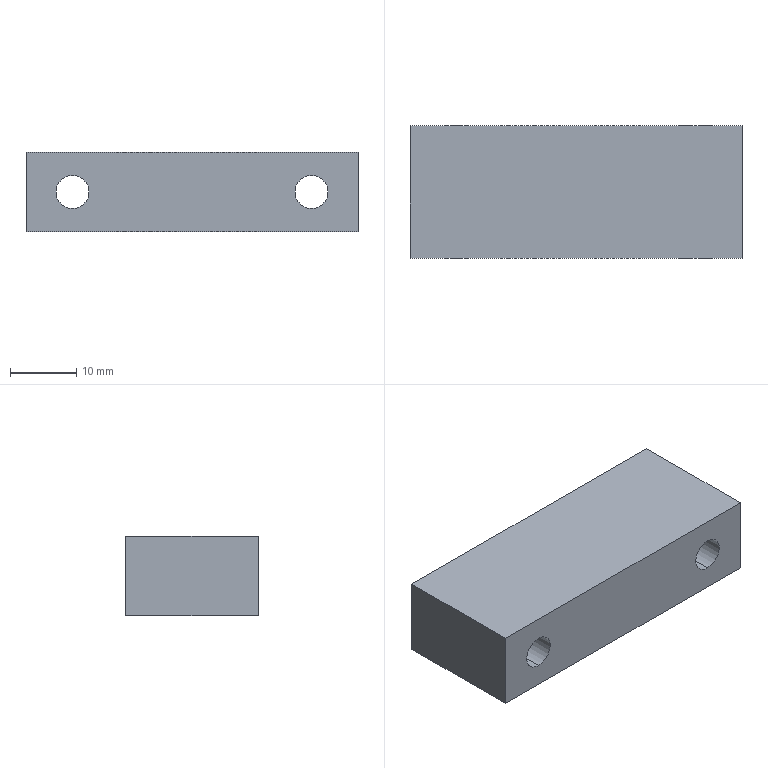Part | STEP file | Cylinder pad plate | 1 solid | 10 faces | box 50 x 20 x 12 mm | volume 11215 mm3 | plane 6 | cylinder 4 | commonest cylinder face diameters 5 x4
STEP:
#1=CARTESIAN_POINT('',(0.,0.,0.));
#2=DIRECTION('',(0.,0.,1.));
#3=DIRECTION('',(1.,0.,0.));
#4=AXIS2_PLACEMENT_3D('',#1,#2,#3);
#5=CARTESIAN_POINT('',(-137.752,17.174,8.5));
#6=VERTEX_POINT('',#5);
#7=CARTESIAN_POINT('',(-137.752,37.174,8.5));
#8=VERTEX_POINT('',#7);
#9=CARTESIAN_POINT('',(-137.752,17.174,8.5));
#10=DIRECTION('',(0.,1.,0.));
#11=VECTOR('',#10,1.);
#12=LINE('',#9,#11);
#13=CARTESIAN_POINT('',(-137.752,17.174,6.));
#14=DIRECTION('',(0.,1.,0.));
#15=DIRECTION('',(0.,0.,1.));
#16=AXIS2_PLACEMENT_3D('',#13,#14,#15);
#17=CYLINDRICAL_SURFACE('',#16,2.5);
#18=CARTESIAN_POINT('',(6.283,0.));
#19=DIRECTION('',(0.,1.));
#20=VECTOR('',#19,1.);
#21=LINE('',#18,#20);
#22=(GEOMETRIC_REPRESENTATION_CONTEXT(2)PARAMETRIC_REPRESENTATION_CONTEXT()REPRESENTATION_CONTEXT('',''));
#23=DEFINITIONAL_REPRESENTATION('',(#21),#22);
#24=PCURVE('',#17,#23);
#25=CARTESIAN_POINT('',(-137.752,17.174,6.));
#26=DIRECTION('',(0.,1.,0.));
#27=DIRECTION('',(0.,0.,1.));
#28=AXIS2_PLACEMENT_3D('',#25,#26,#27);
#29=CYLINDRICAL_SURFACE('',#28,2.5);
#30=CARTESIAN_POINT('',(0.,0.));
#31=DIRECTION('',(0.,1.));
#32=VECTOR('',#31,1.);
#33=LINE('',#30,#32);
#34=(GEOMETRIC_REPRESENTATION_CONTEXT(2)PARAMETRIC_REPRESENTATION_CONTEXT()REPRESENTATION_CONTEXT('',''));
#35=DEFINITIONAL_REPRESENTATION('',(#33),#34);
#36=PCURVE('',#29,#35);
#37=SURFACE_CURVE('',#12,(#24,#36),.PCURVE_S1.);
#38=EDGE_CURVE('',#6,#8,#37,.T.);
#39=ORIENTED_EDGE('',*,*,#38,.T.);
#40=CARTESIAN_POINT('',(-137.752,37.174,3.5));
#41=VERTEX_POINT('',#40);
#42=CARTESIAN_POINT('',(-137.752,37.174,6.));
#43=DIRECTION('',(0.,1.,0.));
#44=DIRECTION('',(0.,0.,1.));
#45=AXIS2_PLACEMENT_3D('',#42,#43,#44);
#46=CIRCLE('',#45,2.5);
#47=CARTESIAN_POINT('',(0.,20.));
#48=DIRECTION('',(1.,0.));
#49=VECTOR('',#48,1.);
#50=LINE('',#47,#49);
#51=(GEOMETRIC_REPRESENTATION_CONTEXT(2)PARAMETRIC_REPRESENTATION_CONTEXT()REPRESENTATION_CONTEXT('',''));
#52=DEFINITIONAL_REPRESENTATION('',(#50),#51);
#53=PCURVE('',#17,#52);
#54=CARTESIAN_POINT('',(-144.752,37.174,12.));
#55=DIRECTION('',(0.,-1.,0.));
#56=DIRECTION('',(0.,0.,-1.));
#57=AXIS2_PLACEMENT_3D('',#54,#55,#56);
#58=PLANE('',#57);
#59=CARTESIAN_POINT('',(3.5,7.));
#60=CARTESIAN_POINT('',(3.5,11.33));
#61=CARTESIAN_POINT('',(7.25,9.165));
#62=CARTESIAN_POINT('',(11.,7.));
#63=CARTESIAN_POINT('',(7.25,4.835));
#64=CARTESIAN_POINT('',(3.5,2.67));
#65=CARTESIAN_POINT('',(3.5,7.));
#66=(BOUNDED_CURVE()B_SPLINE_CURVE(2,(#59,#60,#61,#62,#63,#64,#65),.UNSPECIFIED.,.T.,.F.)B_SPLINE_CURVE_WITH_KNOTS((1,2,2,2,2,1),(-2.094,0.,2.094,4.189,6.283,8.378),.UNSPECIFIED.)CURVE()GEOMETRIC_REPRESENTATION_ITEM()RATIONAL_B_SPLINE_CURVE((1.,0.5,1.,0.5,1.,0.5,1.))REPRESENTATION_ITEM(''));
#67=(GEOMETRIC_REPRESENTATION_CONTEXT(2)PARAMETRIC_REPRESENTATION_CONTEXT()REPRESENTATION_CONTEXT('',''));
#68=DEFINITIONAL_REPRESENTATION('',(#66),#67);
#69=PCURVE('',#58,#68);
#70=SURFACE_CURVE('',#46,(#53,#69),.PCURVE_S1.);
#71=EDGE_CURVE('',#41,#8,#70,.T.);
#72=ORIENTED_EDGE('',*,*,#71,.F.);
#73=CARTESIAN_POINT('',(-137.752,17.174,3.5));
#74=VERTEX_POINT('',#73);
#75=CARTESIAN_POINT('',(-137.752,17.174,3.5));
#76=DIRECTION('',(0.,1.,0.));
#77=VECTOR('',#76,1.);
#78=LINE('',#75,#77);
#79=CARTESIAN_POINT('',(3.142,0.));
#80=DIRECTION('',(0.,1.));
#81=VECTOR('',#80,1.);
#82=LINE('',#79,#81);
#83=(GEOMETRIC_REPRESENTATION_CONTEXT(2)PARAMETRIC_REPRESENTATION_CONTEXT()REPRESENTATION_CONTEXT('',''));
#84=DEFINITIONAL_REPRESENTATION('',(#82),#83);
#85=PCURVE('',#17,#84);
#86=CARTESIAN_POINT('',(3.142,0.));
#87=DIRECTION('',(0.,1.));
#88=VECTOR('',#87,1.);
#89=LINE('',#86,#88);
#90=(GEOMETRIC_REPRESENTATION_CONTEXT(2)PARAMETRIC_REPRESENTATION_CONTEXT()REPRESENTATION_CONTEXT('',''));
#91=DEFINITIONAL_REPRESENTATION('',(#89),#90);
#92=PCURVE('',#29,#91);
#93=SURFACE_CURVE('',#78,(#85,#92),.PCURVE_S1.);
#94=EDGE_CURVE('',#74,#41,#93,.T.);
#95=ORIENTED_EDGE('',*,*,#94,.F.);
#96=CARTESIAN_POINT('',(-137.752,17.174,6.));
#97=DIRECTION('',(0.,1.,0.));
#98=DIRECTION('',(0.,0.,1.));
#99=AXIS2_PLACEMENT_3D('',#96,#97,#98);
#100=CIRCLE('',#99,2.5);
#101=CARTESIAN_POINT('',(0.,0.));
#102=DIRECTION('',(1.,0.));
#103=VECTOR('',#102,1.);
#104=LINE('',#101,#103);
#105=(GEOMETRIC_REPRESENTATION_CONTEXT(2)PARAMETRIC_REPRESENTATION_CONTEXT()REPRESENTATION_CONTEXT('',''));
#106=DEFINITIONAL_REPRESENTATION('',(#104),#105);
#107=PCURVE('',#17,#106);
#108=CARTESIAN_POINT('',(-144.752,17.174,12.));
#109=DIRECTION('',(0.,1.,0.));
#110=DIRECTION('',(0.,0.,1.));
#111=AXIS2_PLACEMENT_3D('',#108,#109,#110);
#112=PLANE('',#111);
#113=CARTESIAN_POINT('',(-6.,7.));
#114=DIRECTION('',(1.,0.));
#115=AXIS2_PLACEMENT_2D('',#113,#114);
#116=CIRCLE('',#115,2.5);
#117=(GEOMETRIC_REPRESENTATION_CONTEXT(2)PARAMETRIC_REPRESENTATION_CONTEXT()REPRESENTATION_CONTEXT('',''));
#118=DEFINITIONAL_REPRESENTATION('',(#116),#117);
#119=PCURVE('',#112,#118);
#120=SURFACE_CURVE('',#100,(#107,#119),.PCURVE_S1.);
#121=EDGE_CURVE('',#74,#6,#120,.T.);
#122=ORIENTED_EDGE('',*,*,#121,.T.);
#123=EDGE_LOOP('',(#39,#72,#95,#122));
#124=FACE_BOUND('',#123,.F.);
#125=ADVANCED_FACE('',(#124),#17,.F.);
#126=CARTESIAN_POINT('',(-101.752,17.174,8.5));
#127=VERTEX_POINT('',#126);
#128=CARTESIAN_POINT('',(-101.752,37.174,8.5));
#129=VERTEX_POINT('',#128);
#130=CARTESIAN_POINT('',(-101.752,17.174,8.5));
#131=DIRECTION('',(0.,1.,0.));
#132=VECTOR('',#131,1.);
#133=LINE('',#130,#132);
#134=CARTESIAN_POINT('',(-101.752,17.174,6.));
#135=DIRECTION('',(0.,1.,0.));
#136=DIRECTION('',(0.,0.,1.));
#137=AXIS2_PLACEMENT_3D('',#134,#135,#136);
#138=CYLINDRICAL_SURFACE('',#137,2.5);
#139=CARTESIAN_POINT('',(6.283,0.));
#140=DIRECTION('',(0.,1.));
#141=VECTOR('',#140,1.);
#142=LINE('',#139,#141);
#143=(GEOMETRIC_REPRESENTATION_CONTEXT(2)PARAMETRIC_REPRESENTATION_CONTEXT()REPRESENTATION_CONTEXT('',''));
#144=DEFINITIONAL_REPRESENTATION('',(#142),#143);
#145=PCURVE('',#138,#144);
#146=CARTESIAN_POINT('',(-101.752,17.174,6.));
#147=DIRECTION('',(0.,1.,0.));
#148=DIRECTION('',(0.,0.,1.));
#149=AXIS2_PLACEMENT_3D('',#146,#147,#148);
#150=CYLINDRICAL_SURFACE('',#149,2.5);
#151=CARTESIAN_POINT('',(0.,0.));
#152=DIRECTION('',(0.,1.));
#153=VECTOR('',#152,1.);
#154=LINE('',#151,#153);
#155=(GEOMETRIC_REPRESENTATION_CONTEXT(2)PARAMETRIC_REPRESENTATION_CONTEXT()REPRESENTATION_CONTEXT('',''));
#156=DEFINITIONAL_REPRESENTATION('',(#154),#155);
#157=PCURVE('',#150,#156);
#158=SURFACE_CURVE('',#133,(#145,#157),.PCURVE_S1.);
#159=EDGE_CURVE('',#127,#129,#158,.T.);
#160=ORIENTED_EDGE('',*,*,#159,.T.);
#161=CARTESIAN_POINT('',(-101.752,37.174,3.5));
#162=VERTEX_POINT('',#161);
#163=CARTESIAN_POINT('',(-101.752,37.174,6.));
#164=DIRECTION('',(0.,1.,0.));
#165=DIRECTION('',(0.,0.,1.));
#166=AXIS2_PLACEMENT_3D('',#163,#164,#165);
#167=CIRCLE('',#166,2.5);
#168=CARTESIAN_POINT('',(0.,20.));
#169=DIRECTION('',(1.,0.));
#170=VECTOR('',#169,1.);
#171=LINE('',#168,#170);
#172=(GEOMETRIC_REPRESENTATION_CONTEXT(2)PARAMETRIC_REPRESENTATION_CONTEXT()REPRESENTATION_CONTEXT('',''));
#173=DEFINITIONAL_REPRESENTATION('',(#171),#172);
#174=PCURVE('',#138,#173);
#175=CARTESIAN_POINT('',(3.5,43.));
#176=CARTESIAN_POINT('',(3.5,47.33));
#177=CARTESIAN_POINT('',(7.25,45.165));
#178=CARTESIAN_POINT('',(11.,43.));
#179=CARTESIAN_POINT('',(7.25,40.835));
#180=CARTESIAN_POINT('',(3.5,38.67));
#181=CARTESIAN_POINT('',(3.5,43.));
#182=(BOUNDED_CURVE()B_SPLINE_CURVE(2,(#175,#176,#177,#178,#179,#180,#181),.UNSPECIFIED.,.T.,.F.)B_SPLINE_CURVE_WITH_KNOTS((1,2,2,2,2,1),(-2.094,0.,2.094,4.189,6.283,8.378),.UNSPECIFIED.)CURVE()GEOMETRIC_REPRESENTATION_ITEM()RATIONAL_B_SPLINE_CURVE((1.,0.5,1.,0.5,1.,0.5,1.))REPRESENTATION_ITEM(''));
#183=(GEOMETRIC_REPRESENTATION_CONTEXT(2)PARAMETRIC_REPRESENTATION_CONTEXT()REPRESENTATION_CONTEXT('',''));
#184=DEFINITIONAL_REPRESENTATION('',(#182),#183);
#185=PCURVE('',#58,#184);
#186=SURFACE_CURVE('',#167,(#174,#185),.PCURVE_S1.);
#187=EDGE_CURVE('',#162,#129,#186,.T.);
#188=ORIENTED_EDGE('',*,*,#187,.F.);
#189=CARTESIAN_POINT('',(-101.752,17.174,3.5));
#190=VERTEX_POINT('',#189);
#191=CARTESIAN_POINT('',(-101.752,17.174,3.5));
#192=DIRECTION('',(0.,1.,0.));
#193=VECTOR('',#192,1.);
#194=LINE('',#191,#193);
#195=CARTESIAN_POINT('',(3.142,0.));
#196=DIRECTION('',(0.,1.));
#197=VECTOR('',#196,1.);
#198=LINE('',#195,#197);
#199=(GEOMETRIC_REPRESENTATION_CONTEXT(2)PARAMETRIC_REPRESENTATION_CONTEXT()REPRESENTATION_CONTEXT('',''));
#200=DEFINITIONAL_REPRESENTATION('',(#198),#199);
#201=PCURVE('',#138,#200);
#202=CARTESIAN_POINT('',(3.142,0.));
#203=DIRECTION('',(0.,1.));
#204=VECTOR('',#203,1.);
#205=LINE('',#202,#204);
#206=(GEOMETRIC_REPRESENTATION_CONTEXT(2)PARAMETRIC_REPRESENTATION_CONTEXT()REPRESENTATION_CONTEXT('',''));
#207=DEFINITIONAL_REPRESENTATION('',(#205),#206);
#208=PCURVE('',#150,#207);
#209=SURFACE_CURVE('',#194,(#201,#208),.PCURVE_S1.);
#210=EDGE_CURVE('',#190,#162,#209,.T.);
#211=ORIENTED_EDGE('',*,*,#210,.F.);
#212=CARTESIAN_POINT('',(-101.752,17.174,6.));
#213=DIRECTION('',(0.,1.,0.));
#214=DIRECTION('',(0.,0.,1.));
#215=AXIS2_PLACEMENT_3D('',#212,#213,#214);
#216=CIRCLE('',#215,2.5);
#217=CARTESIAN_POINT('',(0.,0.));
#218=DIRECTION('',(1.,0.));
#219=VECTOR('',#218,1.);
#220=LINE('',#217,#219);
#221=(GEOMETRIC_REPRESENTATION_CONTEXT(2)PARAMETRIC_REPRESENTATION_CONTEXT()REPRESENTATION_CONTEXT('',''));
#222=DEFINITIONAL_REPRESENTATION('',(#220),#221);
#223=PCURVE('',#138,#222);
#224=CARTESIAN_POINT('',(-6.,43.));
#225=DIRECTION('',(1.,0.));
#226=AXIS2_PLACEMENT_2D('',#224,#225);
#227=CIRCLE('',#226,2.5);
#228=(GEOMETRIC_REPRESENTATION_CONTEXT(2)PARAMETRIC_REPRESENTATION_CONTEXT()REPRESENTATION_CONTEXT('',''));
#229=DEFINITIONAL_REPRESENTATION('',(#227),#228);
#230=PCURVE('',#112,#229);
#231=SURFACE_CURVE('',#216,(#223,#230),.PCURVE_S1.);
#232=EDGE_CURVE('',#190,#127,#231,.T.);
#233=ORIENTED_EDGE('',*,*,#232,.T.);
#234=EDGE_LOOP('',(#160,#188,#211,#233));
#235=FACE_BOUND('',#234,.F.);
#236=ADVANCED_FACE('',(#235),#138,.F.);
#237=CARTESIAN_POINT('',(-94.752,17.174,0.));
#238=VERTEX_POINT('',#237);
#239=CARTESIAN_POINT('',(-94.752,37.174,0.));
#240=VERTEX_POINT('',#239);
#241=CARTESIAN_POINT('',(-94.752,17.174,0.));
#242=DIRECTION('',(0.,1.,0.));
#243=VECTOR('',#242,1.);
#244=LINE('',#241,#243);
#245=CARTESIAN_POINT('',(-94.752,17.174,12.));
#246=DIRECTION('',(-1.,0.,0.));
#247=DIRECTION('',(0.,-1.,0.));
#248=AXIS2_PLACEMENT_3D('',#245,#246,#247);
#249=PLANE('',#248);
#250=CARTESIAN_POINT('',(0.,-12.));
#251=DIRECTION('',(-1.,0.));
#252=VECTOR('',#251,1.);
#253=LINE('',#250,#252);
#254=(GEOMETRIC_REPRESENTATION_CONTEXT(2)PARAMETRIC_REPRESENTATION_CONTEXT()REPRESENTATION_CONTEXT('',''));
#255=DEFINITIONAL_REPRESENTATION('',(#253),#254);
#256=PCURVE('',#249,#255);
#257=CARTESIAN_POINT('',(0.,0.,0.));
#258=DIRECTION('',(0.,0.,-1.));
#259=DIRECTION('',(-1.,0.,0.));
#260=AXIS2_PLACEMENT_3D('',#257,#258,#259);
#261=PLANE('',#260);
#262=CARTESIAN_POINT('',(94.752,17.174));
#263=DIRECTION('',(0.,1.));
#264=VECTOR('',#263,1.);
#265=LINE('',#262,#264);
#266=(GEOMETRIC_REPRESENTATION_CONTEXT(2)PARAMETRIC_REPRESENTATION_CONTEXT()REPRESENTATION_CONTEXT('',''));
#267=DEFINITIONAL_REPRESENTATION('',(#265),#266);
#268=PCURVE('',#261,#267);
#269=SURFACE_CURVE('',#244,(#256,#268),.PCURVE_S1.);
#270=EDGE_CURVE('',#238,#240,#269,.T.);
#271=ORIENTED_EDGE('',*,*,#270,.T.);
#272=CARTESIAN_POINT('',(-94.752,37.174,12.));
#273=VERTEX_POINT('',#272);
#274=CARTESIAN_POINT('',(-94.752,37.174,12.));
#275=DIRECTION('',(0.,0.,-1.));
#276=VECTOR('',#275,1.);
#277=LINE('',#274,#276);
#278=CARTESIAN_POINT('',(-20.,0.));
#279=DIRECTION('',(0.,-1.));
#280=VECTOR('',#279,1.);
#281=LINE('',#278,#280);
#282=(GEOMETRIC_REPRESENTATION_CONTEXT(2)PARAMETRIC_REPRESENTATION_CONTEXT()REPRESENTATION_CONTEXT('',''));
#283=DEFINITIONAL_REPRESENTATION('',(#281),#282);
#284=PCURVE('',#249,#283);
#285=CARTESIAN_POINT('',(0.,50.));
#286=DIRECTION('',(1.,0.));
#287=VECTOR('',#286,1.);
#288=LINE('',#285,#287);
#289=(GEOMETRIC_REPRESENTATION_CONTEXT(2)PARAMETRIC_REPRESENTATION_CONTEXT()REPRESENTATION_CONTEXT('',''));
#290=DEFINITIONAL_REPRESENTATION('',(#288),#289);
#291=PCURVE('',#58,#290);
#292=SURFACE_CURVE('',#277,(#284,#291),.PCURVE_S1.);
#293=EDGE_CURVE('',#273,#240,#292,.T.);
#294=ORIENTED_EDGE('',*,*,#293,.F.);
#295=CARTESIAN_POINT('',(-94.752,17.174,12.));
#296=VERTEX_POINT('',#295);
#297=CARTESIAN_POINT('',(-94.752,17.174,12.));
#298=DIRECTION('',(0.,1.,0.));
#299=VECTOR('',#298,1.);
#300=LINE('',#297,#299);
#301=CARTESIAN_POINT('',(0.,0.));
#302=DIRECTION('',(-1.,0.));
#303=VECTOR('',#302,1.);
#304=LINE('',#301,#303);
#305=(GEOMETRIC_REPRESENTATION_CONTEXT(2)PARAMETRIC_REPRESENTATION_CONTEXT()REPRESENTATION_CONTEXT('',''));
#306=DEFINITIONAL_REPRESENTATION('',(#304),#305);
#307=PCURVE('',#249,#306);
#308=CARTESIAN_POINT('',(0.,0.,12.));
#309=DIRECTION('',(0.,0.,-1.));
#310=DIRECTION('',(-1.,0.,0.));
#311=AXIS2_PLACEMENT_3D('',#308,#309,#310);
#312=PLANE('',#311);
#313=CARTESIAN_POINT('',(94.752,17.174));
#314=DIRECTION('',(0.,1.));
#315=VECTOR('',#314,1.);
#316=LINE('',#313,#315);
#317=(GEOMETRIC_REPRESENTATION_CONTEXT(2)PARAMETRIC_REPRESENTATION_CONTEXT()REPRESENTATION_CONTEXT('',''));
#318=DEFINITIONAL_REPRESENTATION('',(#316),#317);
#319=PCURVE('',#312,#318);
#320=SURFACE_CURVE('',#300,(#307,#319),.PCURVE_S1.);
#321=EDGE_CURVE('',#296,#273,#320,.T.);
#322=ORIENTED_EDGE('',*,*,#321,.F.);
#323=CARTESIAN_POINT('',(-94.752,17.174,12.));
#324=DIRECTION('',(0.,0.,-1.));
#325=VECTOR('',#324,1.);
#326=LINE('',#323,#325);
#327=CARTESIAN_POINT('',(0.,0.));
#328=DIRECTION('',(0.,-1.));
#329=VECTOR('',#328,1.);
#330=LINE('',#327,#329);
#331=(GEOMETRIC_REPRESENTATION_CONTEXT(2)PARAMETRIC_REPRESENTATION_CONTEXT()REPRESENTATION_CONTEXT('',''));
#332=DEFINITIONAL_REPRESENTATION('',(#330),#331);
#333=PCURVE('',#249,#332);
#334=CARTESIAN_POINT('',(0.,50.));
#335=DIRECTION('',(-1.,0.));
#336=VECTOR('',#335,1.);
#337=LINE('',#334,#336);
#338=(GEOMETRIC_REPRESENTATION_CONTEXT(2)PARAMETRIC_REPRESENTATION_CONTEXT()REPRESENTATION_CONTEXT('',''));
#339=DEFINITIONAL_REPRESENTATION('',(#337),#338);
#340=PCURVE('',#112,#339);
#341=SURFACE_CURVE('',#326,(#333,#340),.PCURVE_S1.);
#342=EDGE_CURVE('',#296,#238,#341,.T.);
#343=ORIENTED_EDGE('',*,*,#342,.T.);
#344=EDGE_LOOP('',(#271,#294,#322,#343));
#345=FACE_BOUND('',#344,.T.);
#346=ADVANCED_FACE('',(#345),#249,.F.);
#347=CARTESIAN_POINT('',(-137.752,37.174,6.));
#348=DIRECTION('',(0.,1.,0.));
#349=DIRECTION('',(0.,0.,1.));
#350=AXIS2_PLACEMENT_3D('',#347,#348,#349);
#351=CIRCLE('',#350,2.5);
#352=CARTESIAN_POINT('',(3.5,7.));
#353=CARTESIAN_POINT('',(3.5,11.33));
#354=CARTESIAN_POINT('',(7.25,9.165));
#355=CARTESIAN_POINT('',(11.,7.));
#356=CARTESIAN_POINT('',(7.25,4.835));
#357=CARTESIAN_POINT('',(3.5,2.67));
#358=CARTESIAN_POINT('',(3.5,7.));
#359=(BOUNDED_CURVE()B_SPLINE_CURVE(2,(#352,#353,#354,#355,#356,#357,#358),.UNSPECIFIED.,.T.,.F.)B_SPLINE_CURVE_WITH_KNOTS((1,2,2,2,2,1),(-2.094,0.,2.094,4.189,6.283,8.378),.UNSPECIFIED.)CURVE()GEOMETRIC_REPRESENTATION_ITEM()RATIONAL_B_SPLINE_CURVE((1.,0.5,1.,0.5,1.,0.5,1.))REPRESENTATION_ITEM(''));
#360=(GEOMETRIC_REPRESENTATION_CONTEXT(2)PARAMETRIC_REPRESENTATION_CONTEXT()REPRESENTATION_CONTEXT('',''));
#361=DEFINITIONAL_REPRESENTATION('',(#359),#360);
#362=PCURVE('',#58,#361);
#363=CARTESIAN_POINT('',(0.,20.));
#364=DIRECTION('',(1.,0.));
#365=VECTOR('',#364,1.);
#366=LINE('',#363,#365);
#367=(GEOMETRIC_REPRESENTATION_CONTEXT(2)PARAMETRIC_REPRESENTATION_CONTEXT()REPRESENTATION_CONTEXT('',''));
#368=DEFINITIONAL_REPRESENTATION('',(#366),#367);
#369=PCURVE('',#29,#368);
#370=SURFACE_CURVE('',#351,(#362,#369),.PCURVE_S1.);
#371=EDGE_CURVE('',#8,#41,#370,.T.);
#372=ORIENTED_EDGE('',*,*,#371,.F.);
#373=ORIENTED_EDGE('',*,*,#71,.F.);
#374=EDGE_LOOP('',(#372,#373));
#375=FACE_BOUND('',#374,.T.);
#376=CARTESIAN_POINT('',(-101.752,37.174,6.));
#377=DIRECTION('',(0.,1.,0.));
#378=DIRECTION('',(0.,0.,1.));
#379=AXIS2_PLACEMENT_3D('',#376,#377,#378);
#380=CIRCLE('',#379,2.5);
#381=CARTESIAN_POINT('',(3.5,43.));
#382=CARTESIAN_POINT('',(3.5,47.33));
#383=CARTESIAN_POINT('',(7.25,45.165));
#384=CARTESIAN_POINT('',(11.,43.));
#385=CARTESIAN_POINT('',(7.25,40.835));
#386=CARTESIAN_POINT('',(3.5,38.67));
#387=CARTESIAN_POINT('',(3.5,43.));
#388=(BOUNDED_CURVE()B_SPLINE_CURVE(2,(#381,#382,#383,#384,#385,#386,#387),.UNSPECIFIED.,.T.,.F.)B_SPLINE_CURVE_WITH_KNOTS((1,2,2,2,2,1),(-2.094,0.,2.094,4.189,6.283,8.378),.UNSPECIFIED.)CURVE()GEOMETRIC_REPRESENTATION_ITEM()RATIONAL_B_SPLINE_CURVE((1.,0.5,1.,0.5,1.,0.5,1.))REPRESENTATION_ITEM(''));
#389=(GEOMETRIC_REPRESENTATION_CONTEXT(2)PARAMETRIC_REPRESENTATION_CONTEXT()REPRESENTATION_CONTEXT('',''));
#390=DEFINITIONAL_REPRESENTATION('',(#388),#389);
#391=PCURVE('',#58,#390);
#392=CARTESIAN_POINT('',(0.,20.));
#393=DIRECTION('',(1.,0.));
#394=VECTOR('',#393,1.);
#395=LINE('',#392,#394);
#396=(GEOMETRIC_REPRESENTATION_CONTEXT(2)PARAMETRIC_REPRESENTATION_CONTEXT()REPRESENTATION_CONTEXT('',''));
#397=DEFINITIONAL_REPRESENTATION('',(#395),#396);
#398=PCURVE('',#150,#397);
#399=SURFACE_CURVE('',#380,(#391,#398),.PCURVE_S1.);
#400=EDGE_CURVE('',#129,#162,#399,.T.);
#401=ORIENTED_EDGE('',*,*,#400,.F.);
#402=ORIENTED_EDGE('',*,*,#187,.F.);
#403=EDGE_LOOP('',(#401,#402));
#404=FACE_BOUND('',#403,.T.);
#405=CARTESIAN_POINT('',(-144.752,37.174,0.));
#406=VERTEX_POINT('',#405);
#407=CARTESIAN_POINT('',(-144.752,37.174,0.));
#408=DIRECTION('',(-1.,0.,0.));
#409=VECTOR('',#408,1.);
#410=LINE('',#407,#409);
#411=CARTESIAN_POINT('',(12.,0.));
#412=DIRECTION('',(0.,-1.));
#413=VECTOR('',#412,1.);
#414=LINE('',#411,#413);
#415=(GEOMETRIC_REPRESENTATION_CONTEXT(2)PARAMETRIC_REPRESENTATION_CONTEXT()REPRESENTATION_CONTEXT('',''));
#416=DEFINITIONAL_REPRESENTATION('',(#414),#415);
#417=PCURVE('',#58,#416);
#418=CARTESIAN_POINT('',(144.752,37.174));
#419=DIRECTION('',(1.,0.));
#420=VECTOR('',#419,1.);
#421=LINE('',#418,#420);
#422=(GEOMETRIC_REPRESENTATION_CONTEXT(2)PARAMETRIC_REPRESENTATION_CONTEXT()REPRESENTATION_CONTEXT('',''));
#423=DEFINITIONAL_REPRESENTATION('',(#421),#422);
#424=PCURVE('',#261,#423);
#425=SURFACE_CURVE('',#410,(#417,#424),.PCURVE_S1.);
#426=EDGE_CURVE('',#240,#406,#425,.T.);
#427=ORIENTED_EDGE('',*,*,#426,.T.);
#428=CARTESIAN_POINT('',(-144.752,37.174,12.));
#429=VERTEX_POINT('',#428);
#430=CARTESIAN_POINT('',(-144.752,37.174,12.));
#431=DIRECTION('',(0.,0.,-1.));
#432=VECTOR('',#431,1.);
#433=LINE('',#430,#432);
#434=CARTESIAN_POINT('',(0.,0.));
#435=DIRECTION('',(1.,0.));
#436=VECTOR('',#435,1.);
#437=LINE('',#434,#436);
#438=(GEOMETRIC_REPRESENTATION_CONTEXT(2)PARAMETRIC_REPRESENTATION_CONTEXT()REPRESENTATION_CONTEXT('',''));
#439=DEFINITIONAL_REPRESENTATION('',(#437),#438);
#440=PCURVE('',#58,#439);
#441=CARTESIAN_POINT('',(-144.752,17.174,12.));
#442=DIRECTION('',(1.,0.,0.));
#443=DIRECTION('',(0.,0.,-1.));
#444=AXIS2_PLACEMENT_3D('',#441,#442,#443);
#445=PLANE('',#444);
#446=CARTESIAN_POINT('',(0.,20.));
#447=DIRECTION('',(1.,0.));
#448=VECTOR('',#447,1.);
#449=LINE('',#446,#448);
#450=(GEOMETRIC_REPRESENTATION_CONTEXT(2)PARAMETRIC_REPRESENTATION_CONTEXT()REPRESENTATION_CONTEXT('',''));
#451=DEFINITIONAL_REPRESENTATION('',(#449),#450);
#452=PCURVE('',#445,#451);
#453=SURFACE_CURVE('',#433,(#440,#452),.PCURVE_S1.);
#454=EDGE_CURVE('',#429,#406,#453,.T.);
#455=ORIENTED_EDGE('',*,*,#454,.F.);
#456=CARTESIAN_POINT('',(-144.752,37.174,12.));
#457=DIRECTION('',(-1.,0.,0.));
#458=VECTOR('',#457,1.);
#459=LINE('',#456,#458);
#460=CARTESIAN_POINT('',(0.,0.));
#461=DIRECTION('',(0.,-1.));
#462=VECTOR('',#461,1.);
#463=LINE('',#460,#462);
#464=(GEOMETRIC_REPRESENTATION_CONTEXT(2)PARAMETRIC_REPRESENTATION_CONTEXT()REPRESENTATION_CONTEXT('',''));
#465=DEFINITIONAL_REPRESENTATION('',(#463),#464);
#466=PCURVE('',#58,#465);
#467=CARTESIAN_POINT('',(144.752,37.174));
#468=DIRECTION('',(1.,0.));
#469=VECTOR('',#468,1.);
#470=LINE('',#467,#469);
#471=(GEOMETRIC_REPRESENTATION_CONTEXT(2)PARAMETRIC_REPRESENTATION_CONTEXT()REPRESENTATION_CONTEXT('',''));
#472=DEFINITIONAL_REPRESENTATION('',(#470),#471);
#473=PCURVE('',#312,#472);
#474=SURFACE_CURVE('',#459,(#466,#473),.PCURVE_S1.);
#475=EDGE_CURVE('',#273,#429,#474,.T.);
#476=ORIENTED_EDGE('',*,*,#475,.F.);
#477=ORIENTED_EDGE('',*,*,#293,.T.);
#478=EDGE_LOOP('',(#427,#455,#476,#477));
#479=FACE_BOUND('',#478,.T.);
#480=ADVANCED_FACE('',(#375,#404,#479),#58,.F.);
#481=CARTESIAN_POINT('',(-144.752,17.174,0.));
#482=VERTEX_POINT('',#481);
#483=CARTESIAN_POINT('',(-144.752,17.174,0.));
#484=DIRECTION('',(0.,-1.,0.));
#485=VECTOR('',#484,1.);
#486=LINE('',#483,#485);
#487=CARTESIAN_POINT('',(12.,0.));
#488=DIRECTION('',(0.,-1.));
#489=VECTOR('',#488,1.);
#490=LINE('',#487,#489);
#491=(GEOMETRIC_REPRESENTATION_CONTEXT(2)PARAMETRIC_REPRESENTATION_CONTEXT()REPRESENTATION_CONTEXT('',''));
#492=DEFINITIONAL_REPRESENTATION('',(#490),#491);
#493=PCURVE('',#445,#492);
#494=CARTESIAN_POINT('',(144.752,17.174));
#495=DIRECTION('',(0.,-1.));
#496=VECTOR('',#495,1.);
#497=LINE('',#494,#496);
#498=(GEOMETRIC_REPRESENTATION_CONTEXT(2)PARAMETRIC_REPRESENTATION_CONTEXT()REPRESENTATION_CONTEXT('',''));
#499=DEFINITIONAL_REPRESENTATION('',(#497),#498);
#500=PCURVE('',#261,#499);
#501=SURFACE_CURVE('',#486,(#493,#500),.PCURVE_S1.);
#502=EDGE_CURVE('',#406,#482,#501,.T.);
#503=ORIENTED_EDGE('',*,*,#502,.T.);
#504=CARTESIAN_POINT('',(-144.752,17.174,12.));
#505=VERTEX_POINT('',#504);
#506=CARTESIAN_POINT('',(-144.752,17.174,12.));
#507=DIRECTION('',(0.,0.,-1.));
#508=VECTOR('',#507,1.);
#509=LINE('',#506,#508);
#510=CARTESIAN_POINT('',(0.,0.));
#511=DIRECTION('',(1.,0.));
#512=VECTOR('',#511,1.);
#513=LINE('',#510,#512);
#514=(GEOMETRIC_REPRESENTATION_CONTEXT(2)PARAMETRIC_REPRESENTATION_CONTEXT()REPRESENTATION_CONTEXT('',''));
#515=DEFINITIONAL_REPRESENTATION('',(#513),#514);
#516=PCURVE('',#445,#515);
#517=CARTESIAN_POINT('',(0.,0.));
#518=DIRECTION('',(-1.,0.));
#519=VECTOR('',#518,1.);
#520=LINE('',#517,#519);
#521=(GEOMETRIC_REPRESENTATION_CONTEXT(2)PARAMETRIC_REPRESENTATION_CONTEXT()REPRESENTATION_CONTEXT('',''));
#522=DEFINITIONAL_REPRESENTATION('',(#520),#521);
#523=PCURVE('',#112,#522);
#524=SURFACE_CURVE('',#509,(#516,#523),.PCURVE_S1.);
#525=EDGE_CURVE('',#505,#482,#524,.T.);
#526=ORIENTED_EDGE('',*,*,#525,.F.);
#527=CARTESIAN_POINT('',(-144.752,17.174,12.));
#528=DIRECTION('',(0.,-1.,0.));
#529=VECTOR('',#528,1.);
#530=LINE('',#527,#529);
#531=CARTESIAN_POINT('',(0.,0.));
#532=DIRECTION('',(0.,-1.));
#533=VECTOR('',#532,1.);
#534=LINE('',#531,#533);
#535=(GEOMETRIC_REPRESENTATION_CONTEXT(2)PARAMETRIC_REPRESENTATION_CONTEXT()REPRESENTATION_CONTEXT('',''));
#536=DEFINITIONAL_REPRESENTATION('',(#534),#535);
#537=PCURVE('',#445,#536);
#538=CARTESIAN_POINT('',(144.752,17.174));
#539=DIRECTION('',(0.,-1.));
#540=VECTOR('',#539,1.);
#541=LINE('',#538,#540);
#542=(GEOMETRIC_REPRESENTATION_CONTEXT(2)PARAMETRIC_REPRESENTATION_CONTEXT()REPRESENTATION_CONTEXT('',''));
#543=DEFINITIONAL_REPRESENTATION('',(#541),#542);
#544=PCURVE('',#312,#543);
#545=SURFACE_CURVE('',#530,(#537,#544),.PCURVE_S1.);
#546=EDGE_CURVE('',#429,#505,#545,.T.);
#547=ORIENTED_EDGE('',*,*,#546,.F.);
#548=ORIENTED_EDGE('',*,*,#454,.T.);
#549=EDGE_LOOP('',(#503,#526,#547,#548));
#550=FACE_BOUND('',#549,.T.);
#551=ADVANCED_FACE('',(#550),#445,.F.);
#552=CARTESIAN_POINT('',(-137.752,17.174,6.));
#553=DIRECTION('',(0.,1.,0.));
#554=DIRECTION('',(0.,0.,1.));
#555=AXIS2_PLACEMENT_3D('',#552,#553,#554);
#556=CIRCLE('',#555,2.5);
#557=CARTESIAN_POINT('',(-6.,7.));
#558=DIRECTION('',(1.,0.));
#559=AXIS2_PLACEMENT_2D('',#557,#558);
#560=CIRCLE('',#559,2.5);
#561=(GEOMETRIC_REPRESENTATION_CONTEXT(2)PARAMETRIC_REPRESENTATION_CONTEXT()REPRESENTATION_CONTEXT('',''));
#562=DEFINITIONAL_REPRESENTATION('',(#560),#561);
#563=PCURVE('',#112,#562);
#564=CARTESIAN_POINT('',(0.,0.));
#565=DIRECTION('',(1.,0.));
#566=VECTOR('',#565,1.);
#567=LINE('',#564,#566);
#568=(GEOMETRIC_REPRESENTATION_CONTEXT(2)PARAMETRIC_REPRESENTATION_CONTEXT()REPRESENTATION_CONTEXT('',''));
#569=DEFINITIONAL_REPRESENTATION('',(#567),#568);
#570=PCURVE('',#29,#569);
#571=SURFACE_CURVE('',#556,(#563,#570),.PCURVE_S1.);
#572=EDGE_CURVE('',#6,#74,#571,.T.);
#573=ORIENTED_EDGE('',*,*,#572,.T.);
#574=ORIENTED_EDGE('',*,*,#121,.T.);
#575=EDGE_LOOP('',(#573,#574));
#576=FACE_BOUND('',#575,.T.);
#577=CARTESIAN_POINT('',(-101.752,17.174,6.));
#578=DIRECTION('',(0.,1.,0.));
#579=DIRECTION('',(0.,0.,1.));
#580=AXIS2_PLACEMENT_3D('',#577,#578,#579);
#581=CIRCLE('',#580,2.5);
#582=CARTESIAN_POINT('',(-6.,43.));
#583=DIRECTION('',(1.,0.));
#584=AXIS2_PLACEMENT_2D('',#582,#583);
#585=CIRCLE('',#584,2.5);
#586=(GEOMETRIC_REPRESENTATION_CONTEXT(2)PARAMETRIC_REPRESENTATION_CONTEXT()REPRESENTATION_CONTEXT('',''));
#587=DEFINITIONAL_REPRESENTATION('',(#585),#586);
#588=PCURVE('',#112,#587);
#589=CARTESIAN_POINT('',(0.,0.));
#590=DIRECTION('',(1.,0.));
#591=VECTOR('',#590,1.);
#592=LINE('',#589,#591);
#593=(GEOMETRIC_REPRESENTATION_CONTEXT(2)PARAMETRIC_REPRESENTATION_CONTEXT()REPRESENTATION_CONTEXT('',''));
#594=DEFINITIONAL_REPRESENTATION('',(#592),#593);
#595=PCURVE('',#150,#594);
#596=SURFACE_CURVE('',#581,(#588,#595),.PCURVE_S1.);
#597=EDGE_CURVE('',#127,#190,#596,.T.);
#598=ORIENTED_EDGE('',*,*,#597,.T.);
#599=ORIENTED_EDGE('',*,*,#232,.T.);
#600=EDGE_LOOP('',(#598,#599));
#601=FACE_BOUND('',#600,.T.);
#602=CARTESIAN_POINT('',(-144.752,17.174,0.));
#603=DIRECTION('',(1.,0.,0.));
#604=VECTOR('',#603,1.);
#605=LINE('',#602,#604);
#606=CARTESIAN_POINT('',(-12.,0.));
#607=DIRECTION('',(0.,1.));
#608=VECTOR('',#607,1.);
#609=LINE('',#606,#608);
#610=(GEOMETRIC_REPRESENTATION_CONTEXT(2)PARAMETRIC_REPRESENTATION_CONTEXT()REPRESENTATION_CONTEXT('',''));
#611=DEFINITIONAL_REPRESENTATION('',(#609),#610);
#612=PCURVE('',#112,#611);
#613=CARTESIAN_POINT('',(144.752,17.174));
#614=DIRECTION('',(-1.,0.));
#615=VECTOR('',#614,1.);
#616=LINE('',#613,#615);
#617=(GEOMETRIC_REPRESENTATION_CONTEXT(2)PARAMETRIC_REPRESENTATION_CONTEXT()REPRESENTATION_CONTEXT('',''));
#618=DEFINITIONAL_REPRESENTATION('',(#616),#617);
#619=PCURVE('',#261,#618);
#620=SURFACE_CURVE('',#605,(#612,#619),.PCURVE_S1.);
#621=EDGE_CURVE('',#482,#238,#620,.T.);
#622=ORIENTED_EDGE('',*,*,#621,.T.);
#623=ORIENTED_EDGE('',*,*,#342,.F.);
#624=CARTESIAN_POINT('',(-144.752,17.174,12.));
#625=DIRECTION('',(1.,0.,0.));
#626=VECTOR('',#625,1.);
#627=LINE('',#624,#626);
#628=CARTESIAN_POINT('',(0.,0.));
#629=DIRECTION('',(0.,1.));
#630=VECTOR('',#629,1.);
#631=LINE('',#628,#630);
#632=(GEOMETRIC_REPRESENTATION_CONTEXT(2)PARAMETRIC_REPRESENTATION_CONTEXT()REPRESENTATION_CONTEXT('',''));
#633=DEFINITIONAL_REPRESENTATION('',(#631),#632);
#634=PCURVE('',#112,#633);
#635=CARTESIAN_POINT('',(144.752,17.174));
#636=DIRECTION('',(-1.,0.));
#637=VECTOR('',#636,1.);
#638=LINE('',#635,#637);
#639=(GEOMETRIC_REPRESENTATION_CONTEXT(2)PARAMETRIC_REPRESENTATION_CONTEXT()REPRESENTATION_CONTEXT('',''));
#640=DEFINITIONAL_REPRESENTATION('',(#638),#639);
#641=PCURVE('',#312,#640);
#642=SURFACE_CURVE('',#627,(#634,#641),.PCURVE_S1.);
#643=EDGE_CURVE('',#505,#296,#642,.T.);
#644=ORIENTED_EDGE('',*,*,#643,.F.);
#645=ORIENTED_EDGE('',*,*,#525,.T.);
#646=EDGE_LOOP('',(#622,#623,#644,#645));
#647=FACE_BOUND('',#646,.T.);
#648=ADVANCED_FACE('',(#576,#601,#647),#112,.F.);
#649=ORIENTED_EDGE('',*,*,#321,.T.);
#650=ORIENTED_EDGE('',*,*,#475,.T.);
#651=ORIENTED_EDGE('',*,*,#546,.T.);
#652=ORIENTED_EDGE('',*,*,#643,.T.);
#653=EDGE_LOOP('',(#649,#650,#651,#652));
#654=FACE_BOUND('',#653,.T.);
#655=ADVANCED_FACE('',(#654),#312,.F.);
#656=ORIENTED_EDGE('',*,*,#270,.F.);
#657=ORIENTED_EDGE('',*,*,#621,.F.);
#658=ORIENTED_EDGE('',*,*,#502,.F.);
#659=ORIENTED_EDGE('',*,*,#426,.F.);
#660=EDGE_LOOP('',(#656,#657,#658,#659));
#661=FACE_BOUND('',#660,.T.);
#662=ADVANCED_FACE('',(#661),#261,.T.);
#663=ORIENTED_EDGE('',*,*,#400,.F.);
#664=ORIENTED_EDGE('',*,*,#159,.F.);
#665=ORIENTED_EDGE('',*,*,#597,.T.);
#666=ORIENTED_EDGE('',*,*,#210,.T.);
#667=EDGE_LOOP('',(#663,#664,#665,#666));
#668=FACE_BOUND('',#667,.F.);
#669=ADVANCED_FACE('',(#668),#150,.F.);
#670=ORIENTED_EDGE('',*,*,#371,.F.);
#671=ORIENTED_EDGE('',*,*,#38,.F.);
#672=ORIENTED_EDGE('',*,*,#572,.T.);
#673=ORIENTED_EDGE('',*,*,#94,.T.);
#674=EDGE_LOOP('',(#670,#671,#672,#673));
#675=FACE_BOUND('',#674,.F.);
#676=ADVANCED_FACE('',(#675),#29,.F.);
#677=CLOSED_SHELL('',(#125,#236,#346,#480,#551,#648,#655,#662,#669,#676));
#678=MANIFOLD_SOLID_BREP('',#677);
#679=(LENGTH_UNIT()NAMED_UNIT(*)SI_UNIT(.MILLI.,.METRE.));
#680=UNCERTAINTY_MEASURE_WITH_UNIT(LENGTH_MEASURE(0.0000001),#679,'','');
#681=(NAMED_UNIT(*)PLANE_ANGLE_UNIT()SI_UNIT($,.RADIAN.));
#682=(NAMED_UNIT(*)SI_UNIT($,.STERADIAN.)SOLID_ANGLE_UNIT());
#683=(GEOMETRIC_REPRESENTATION_CONTEXT(3)GLOBAL_UNCERTAINTY_ASSIGNED_CONTEXT((#680))GLOBAL_UNIT_ASSIGNED_CONTEXT((#679,#681,#682))REPRESENTATION_CONTEXT('',''));
#684=ADVANCED_BREP_SHAPE_REPRESENTATION('',(#4,#678),#683);